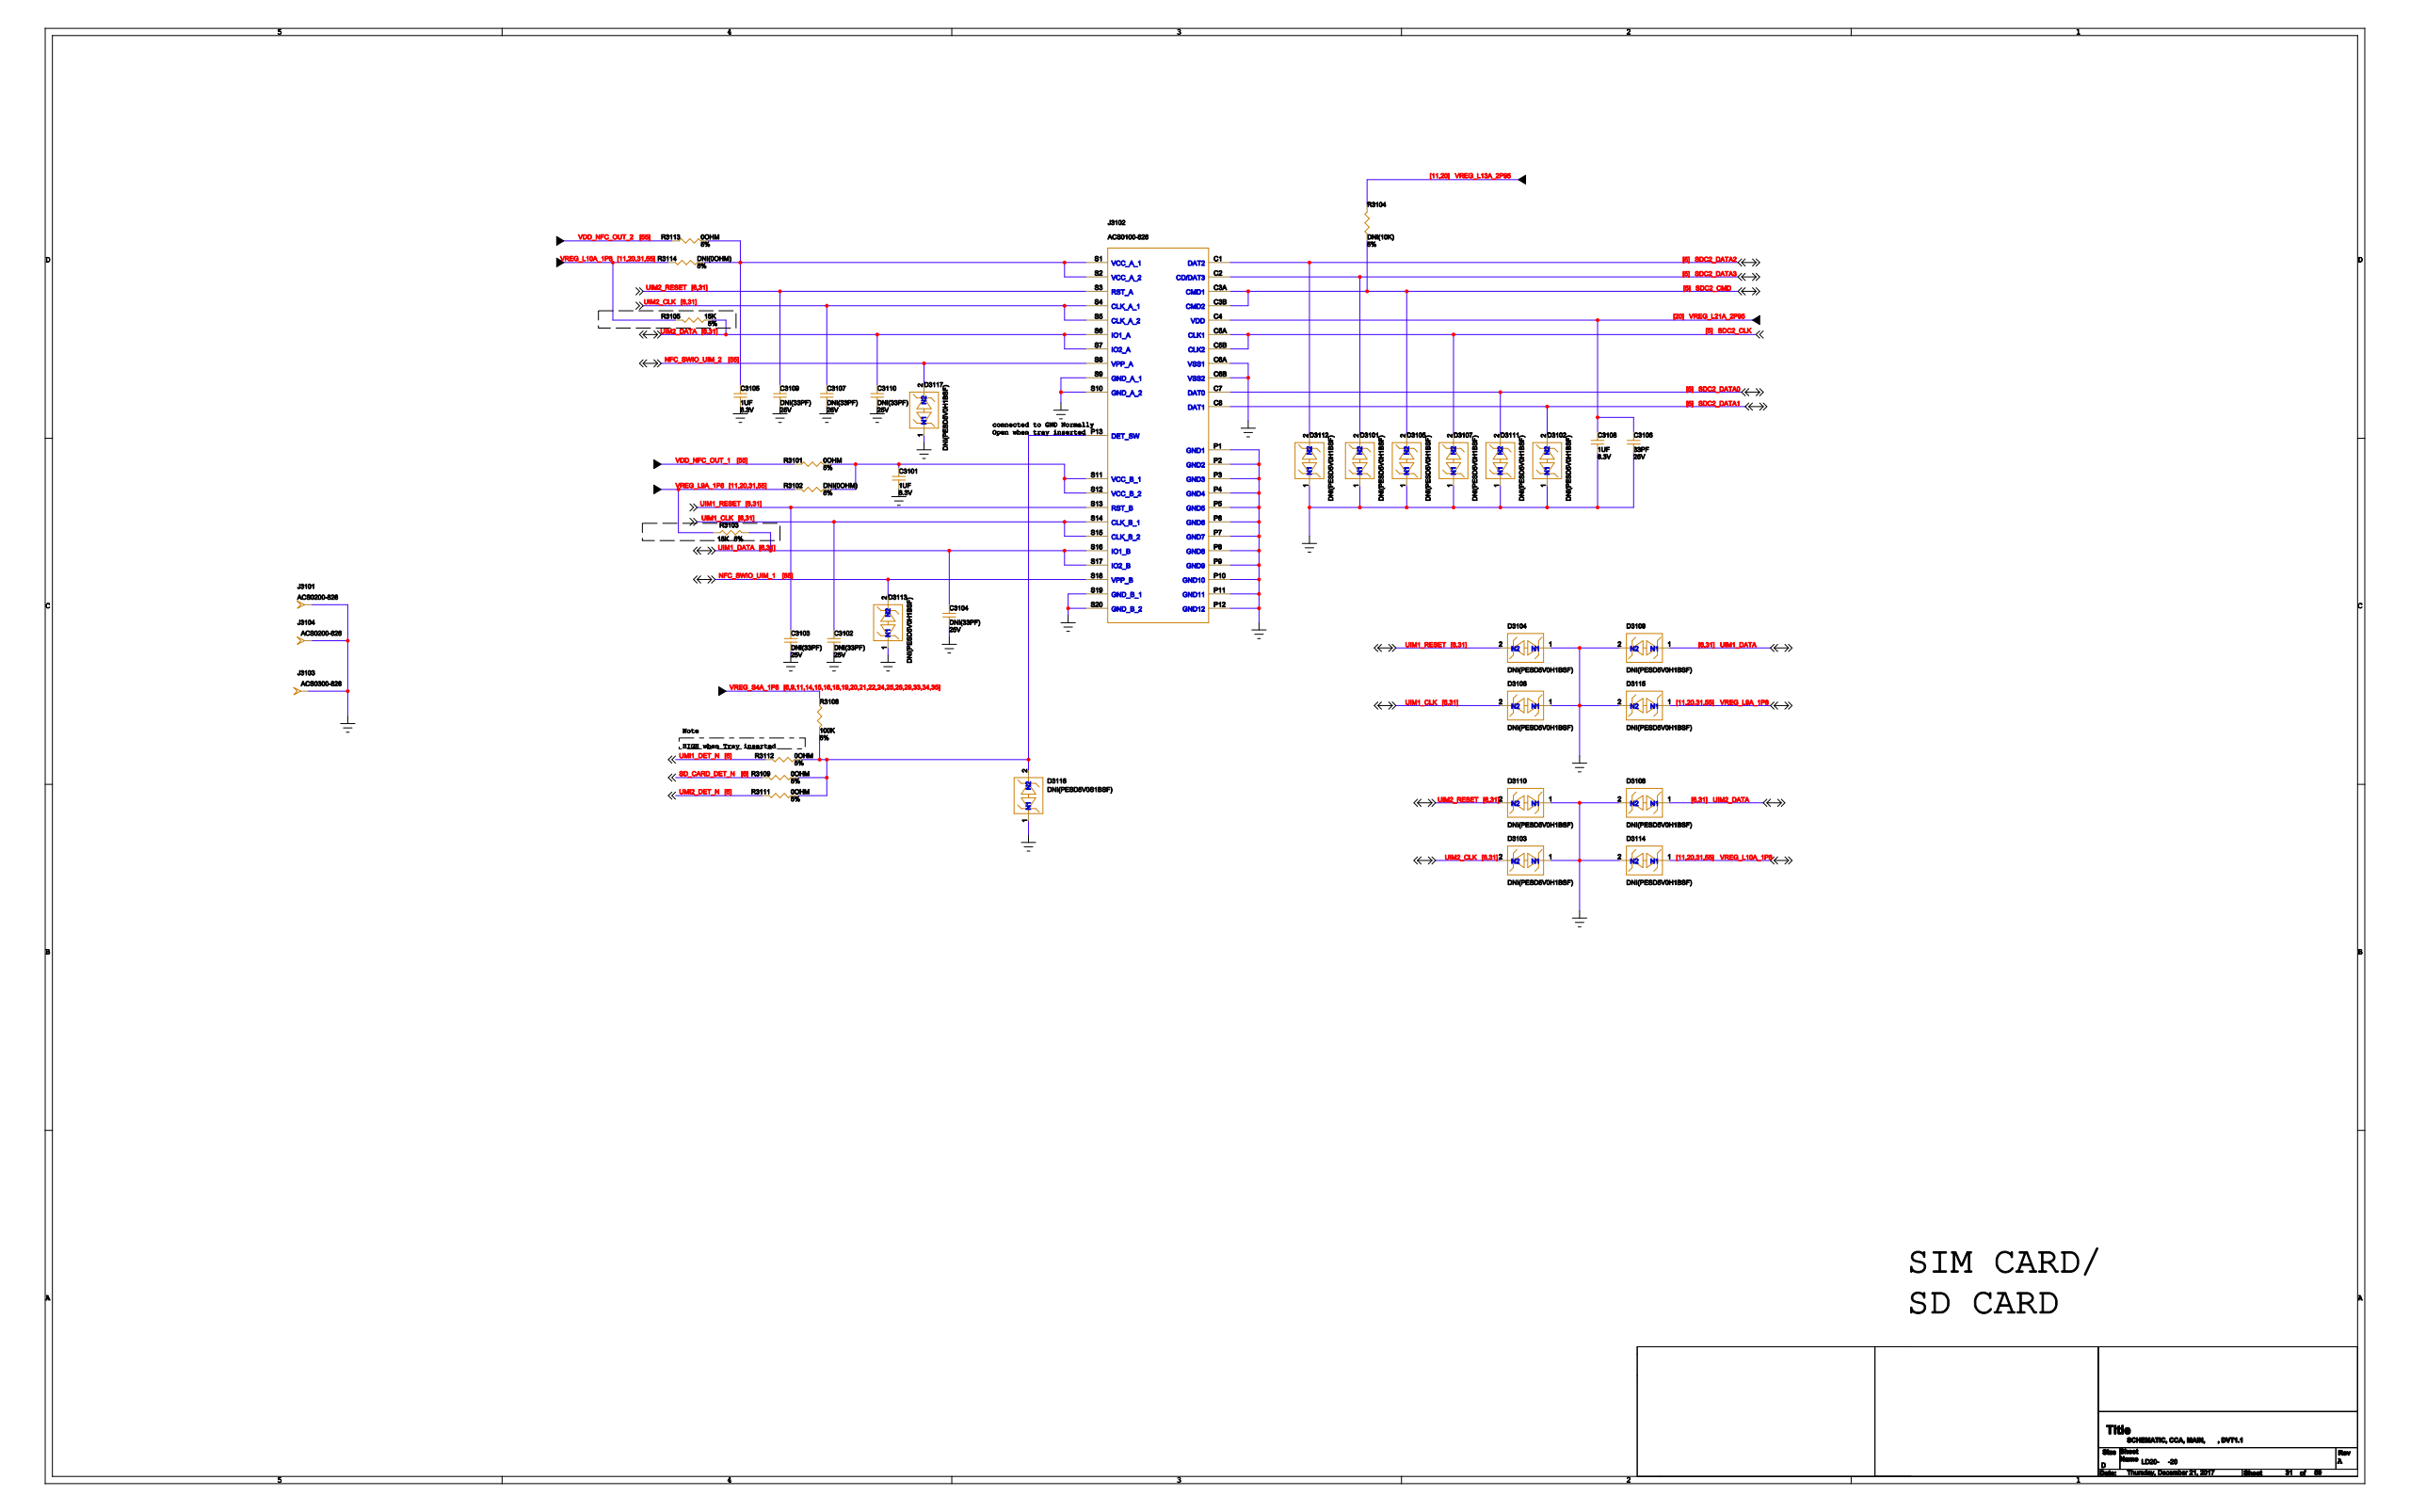Circuit board | Cadence Allegro | 1520 parts | 1149 nets | one sheet of the schematic
Parts on this sheet (reference | value | footprint):
C3101 | 1UF | 2P0201R
C3102 | DNI(33PF) | 2P0201R_DNI
C3103 | DNI(33PF) | 2P0201R_DNI
C3104 | DNI(33PF) | 2P0201R_DNI
C3105 | 1UF | 2P0201R
C3106 | 33PF | 2P0201R
C3107 | DNI(33PF) | 2P0201R_DNI
C3108 | 1UF | 2P0201R
C3109 | DNI(33PF) | 2P0201R_DNI
C3110 | DNI(33PF) | 2P0201R_DNI
D3101 | DNI(PESD5V0H1BSF) | 2PSM25X13N_DNI
D3102 | DNI(PESD5V0H1BSF) | 2PSM25X13N_DNI
D3103 | DNI(PESD5V0H1BSF) | 2PSM25X13N_DNI
D3104 | DNI(PESD5V0H1BSF) | 2PSM25X13N_DNI
D3105 | DNI(PESD5V0H1BSF) | 2PSM25X13N_DNI
D3106 | DNI(PESD5V0H1BSF) | 2PSM25X13N_DNI
D3107 | DNI(PESD5V0H1BSF) | 2PSM25X13N_DNI
D3108 | DNI(PESD5V0H1BSF) | 2PSM25X13N_DNI
D3109 | DNI(PESD5V0H1BSF) | 2PSM25X13N_DNI
D3110 | DNI(PESD5V0H1BSF) | 2PSM25X13N_DNI
D3111 | DNI(PESD5V0H1BSF) | 2PSM25X13N_DNI
D3112 | DNI(PESD5V0H1BSF) | 2PSM25X13N_DNI
D3113 | DNI(PESD5V0H1BSF) | 2PSM25X13N_DNI
D3114 | DNI(PESD5V0H1BSF) | 2PSM25X13N_DNI
D3115 | DNI(PESD5V0H1BSF) | 2PSM25X13N_DNI
D3116 | DNI(PESD5V0S1BSF) | 2PSM25X13N_DNI
D3117 | DNI(PESD5V0H1BSF) | 2PSM25X13N_DNI
J3101 | ACS0200-826 | TP-0_075
J3102 | ACS0100-826 | 44SCONSRA
J3103 | ACS0300-826 | TP-0_075
J3104 | ACS0200-826 | TP-0_075
R3101 | 0OHM | 2P0201R
R3102 | DNI(0OHM) | 2P0201R_DNI
R3103 | 15K | 2P0201R
R3104 | DNI(10K) | 2P0201R_DNI
R3105 | 15K | 2P0201R
R3106 | 100K | 2P0201R
R3109 | 0OHM | 2P0201R
R3111 | 0OHM | 2P0201R
R3112 | 0OHM | 2P0201R
R3113 | 0OHM | 2P0201R
R3114 | DNI(0OHM) | 2P0201R_DNI
Nets of these parts (net: part-pin ...):
GND: C3101-2 C3102-2 C3103-2 C3104-2 C3105-2 C3106-2 C3107-2 C3108-2 C3109-2 C3110-2 D3101-1 D3102-1 D3103-1 D3104-1 D3105-1 D3106-1 D3107-1 D3108-2 D3109-2 D3110-1 D3111-1 D3112-1 D3113-1 D3114-2 D3115-2 D3116-1 D3117-1 J3101-1 J3103-1 J3104-1 J3102-C6A J3102-C6B J3102-P1 J3102-P2 J3102-P3 J3102-P4 J3102-P5 J3102-P6 J3102-P7 J3102-P8 J3102-P9 J3102-P10 J3102-P11 J3102-P12 J3102-S9 J3102-S10 J3102-S19 J3102-S20
VREG_S4A_1P8: R3106-2
NFC_SWIO_UIM_1: D3113-2 J3102-S18
NFC_SWIO_UIM_2: D3117-2 J3102-S8
VDD_NFC_OUT_1: R3101-2
VDD_NFC_OUT_2: R3113-2
VREG_L9A_1P8: D3115-1 R3102-1 R3103-2
VREG_L10A_1P8: D3114-1 R3105-1 R3114-1
SDC2_DATA3: D3101-2 J3102-C2
SDC2_DATA1: D3102-2 J3102-C8
UIM2_CLK: C3107-1 D3103-2 J3102-S4 J3102-S5
UIM1_RESET: C3103-1 D3104-2 J3102-S13
SDC2_CMD: D3105-2 R3104-2 J3102-C3A J3102-C3B
UIM1_CLK: C3102-1 D3106-2 J3102-S14 J3102-S15
SDC2_CLK: D3107-2 J3102-C5A J3102-C5B
UIM2_DATA: C3110-1 D3108-1 R3105-2 J3102-S6 J3102-S7
UIM1_DATA: C3104-1 D3109-1 R3103-1 J3102-S16 J3102-S17
UIM2_RESET: C3109-1 D3110-2 J3102-S3
SDC2_DATA0: D3111-2 J3102-C7
SDC2_DATA2: D3112-2 J3102-C1
N35375628: D3116-2 R3106-1 R3109-2 R3111-2 R3112-2 J3102-P13
VREG_L13A_2P95: R3104-1
N35374834: C3101-1 R3101-1 R3102-2 J3102-S11 J3102-S12
N35372594: C3105-1 R3113-1 R3114-2 J3102-S1 J3102-S2
VREG_L21A_2P95: C3106-1 C3108-1 J3102-C4
SD_CARD_DET_N: R3109-1
UMI2_DET_N: R3111-1
UMI1_DET_N: R3112-1